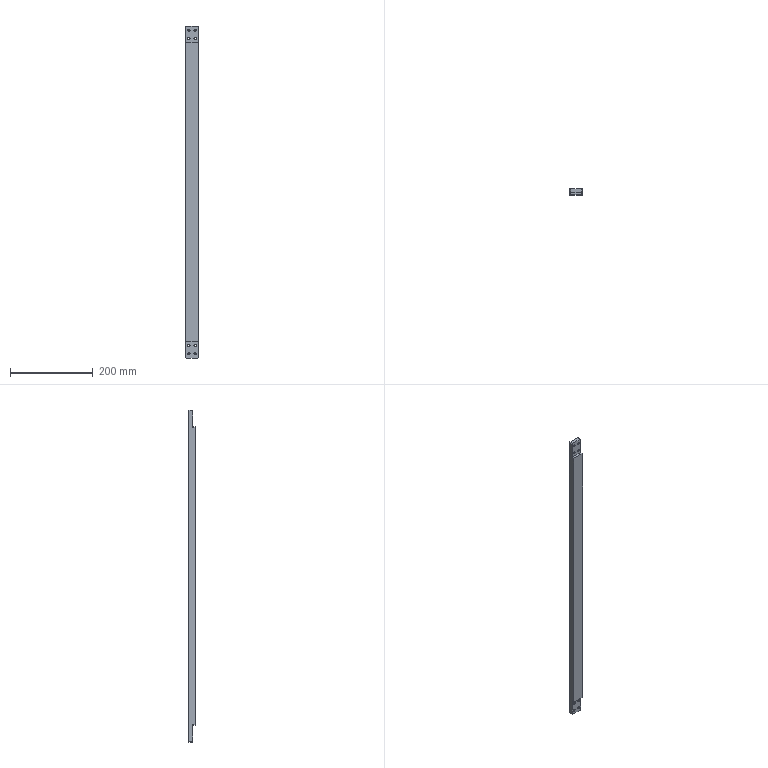Part | SolidWorks | features BaseBody 1 | 1 solid | 58 faces | box 30 x 15 x 801 mm | volume 341853 mm3 | cylinder 32 | plane 26 | commonest cylinder face diameters 5.5 x16 10 x16